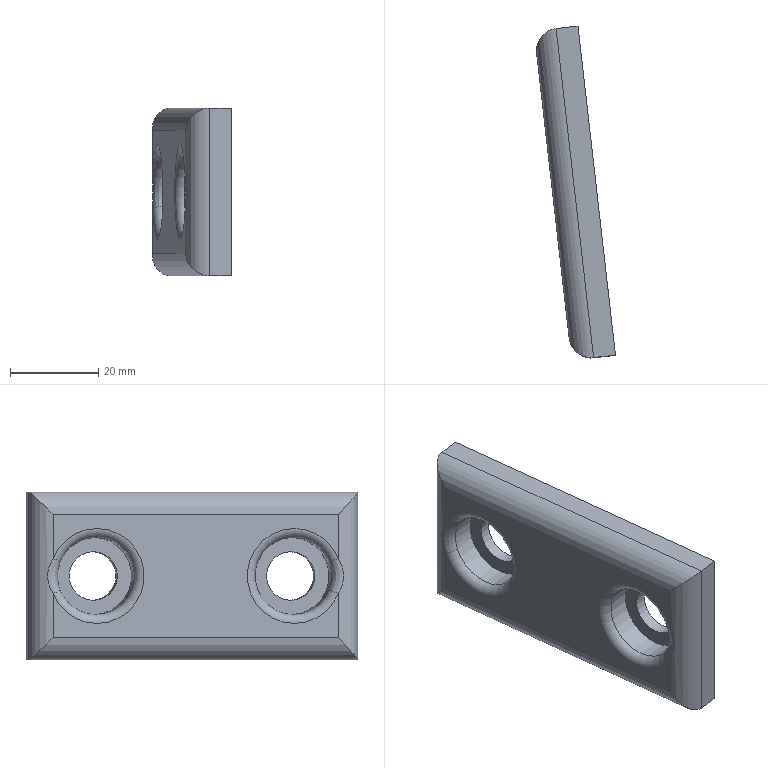Part | NX | features XQ 2 | 1 solid | 20 faces | box 17.898 x 75.116 x 38 mm | volume 23209 mm3 | plane 8 | cylinder 8 | spline 2 | torus 2 | commonest cylinder face diameters 10 x4 11 x2 17.5 x2
STEP:
#1=CARTESIAN_POINT('',(2876.788,318.77,-57.945));
#2=VERTEX_POINT('',#1);
#3=CARTESIAN_POINT('',(2876.788,318.77,-50.055));
#4=VERTEX_POINT('',#3);
#5=CARTESIAN_POINT('',(2876.788,318.77,-50.055));
#6=CARTESIAN_POINT('',(2876.883,317.934,-51.336));
#7=CARTESIAN_POINT('',(2877.291,317.159,-54.001));
#8=CARTESIAN_POINT('',(2876.883,317.934,-56.664));
#9=CARTESIAN_POINT('',(2876.788,318.77,-57.945));
#10=B_SPLINE_CURVE_WITH_KNOTS('',3,(#5,#6,#7,#8,#9),.UNSPECIFIED.,.F.,.F.,(4,1,4),(0.,0.5,1.),.UNSPECIFIED.);
#11=EDGE_CURVE('',#2,#4,#10,.F.);
#12=ORIENTED_EDGE('',*,*,#11,.T.);
#13=CARTESIAN_POINT('',(2878.565,320.845,-50.789));
#14=VERTEX_POINT('',#13);
#15=CARTESIAN_POINT('',(2878.775,318.997,-50.055));
#16=DIRECTION('',(0.04154,-0.3646,-0.9302));
#17=DIRECTION('',(0.,0.931,-0.3649));
#18=AXIS2_PLACEMENT_3D('',#15,#16,#17);
#19=CIRCLE('',#18,2.);
#20=EDGE_CURVE('',#4,#14,#19,.T.);
#21=ORIENTED_EDGE('',*,*,#20,.T.);
#22=CARTESIAN_POINT('',(2878.565,320.845,-57.211));
#23=VERTEX_POINT('',#22);
#24=CARTESIAN_POINT('',(2878.565,320.845,-57.211));
#25=CARTESIAN_POINT('',(2878.572,320.778,-57.039));
#26=CARTESIAN_POINT('',(2878.597,320.624,-56.62));
#27=CARTESIAN_POINT('',(2878.666,320.375,-55.639));
#28=CARTESIAN_POINT('',(2878.721,320.257,-54.616));
#29=CARTESIAN_POINT('',(2878.732,320.246,-54.002));
#30=CARTESIAN_POINT('',(2878.721,320.257,-53.387));
#31=CARTESIAN_POINT('',(2878.666,320.374,-52.363));
#32=CARTESIAN_POINT('',(2878.597,320.624,-51.379));
#33=CARTESIAN_POINT('',(2878.572,320.778,-50.96));
#34=CARTESIAN_POINT('',(2878.565,320.845,-50.789));
#35=B_SPLINE_CURVE_WITH_KNOTS('',3,(#24,#25,#26,#27,#28,#29,#30,#31,#32,#33,#34),.UNSPECIFIED.,.F.,.F.,(4,1,1,1,1,1,1,1,4),(0.,0.125,0.25,0.375,0.5,0.625,0.75,0.875,1.),.UNSPECIFIED.);
#36=EDGE_CURVE('',#14,#23,#35,.F.);
#37=ORIENTED_EDGE('',*,*,#36,.T.);
#38=CARTESIAN_POINT('',(2878.775,318.997,-57.945));
#39=DIRECTION('',(0.04154,-0.3646,0.9302));
#40=DIRECTION('',(0.,0.931,0.3649));
#41=AXIS2_PLACEMENT_3D('',#38,#39,#40);
#42=CIRCLE('',#41,2.);
#43=EDGE_CURVE('',#23,#2,#42,.T.);
#44=ORIENTED_EDGE('',*,*,#43,.T.);
#45=EDGE_LOOP('',(#12,#21,#37,#44));
#46=FACE_BOUND('',#45,.T.);
#47=CARTESIAN_POINT('',(2878.565,320.845,-50.789));
#48=CARTESIAN_POINT('',(2876.577,320.619,-50.789));
#49=CARTESIAN_POINT('',(2876.788,318.77,-50.055));
#50=CARTESIAN_POINT('',(2878.61,320.445,-51.812));
#51=CARTESIAN_POINT('',(2876.298,320.092,-52.036));
#52=CARTESIAN_POINT('',(2876.882,317.95,-51.311));
#53=CARTESIAN_POINT('',(2878.728,320.25,-52.902));
#54=CARTESIAN_POINT('',(2876.163,319.957,-52.986));
#55=CARTESIAN_POINT('',(2877.087,317.547,-52.652));
#56=CARTESIAN_POINT('',(2878.728,320.25,-55.096));
#57=CARTESIAN_POINT('',(2876.163,319.957,-55.012));
#58=CARTESIAN_POINT('',(2877.087,317.546,-55.346));
#59=CARTESIAN_POINT('',(2878.61,320.446,-56.192));
#60=CARTESIAN_POINT('',(2876.299,320.094,-55.968));
#61=CARTESIAN_POINT('',(2876.881,317.952,-56.693));
#62=CARTESIAN_POINT('',(2878.565,320.845,-57.211));
#63=CARTESIAN_POINT('',(2876.577,320.619,-57.211));
#64=CARTESIAN_POINT('',(2876.788,318.77,-57.945));
#65=(BOUNDED_SURFACE()B_SPLINE_SURFACE(3,2,((#47,#48,#49),(#50,#51,#52),(#53,#54,#55),(#56,#57,#58),(#59,#60,#61),(#62,#63,#64)),.UNSPECIFIED.,.F.,.F.,.F.)B_SPLINE_SURFACE_WITH_KNOTS((4,2,4),(3,3),(0.,0.5,1.),(0.,1.),.UNSPECIFIED.)GEOMETRIC_REPRESENTATION_ITEM()RATIONAL_B_SPLINE_SURFACE(((1.,0.7071,1.),(1.,0.6518,1.),(1.,0.6124,1.),(1.,0.6124,1.),(1.,0.6519,1.),(1.,0.7071,1.)))REPRESENTATION_ITEM('')SURFACE());
#66=ADVANCED_FACE('',(#46),#65,.T.);
#67=CARTESIAN_POINT('',(2869.43,383.353,-50.055));
#68=VERTEX_POINT('',#67);
#69=CARTESIAN_POINT('',(2869.43,383.353,-57.945));
#70=VERTEX_POINT('',#69);
#71=CARTESIAN_POINT('',(2869.43,383.353,-57.945));
#72=CARTESIAN_POINT('',(2869.335,384.189,-56.664));
#73=CARTESIAN_POINT('',(2869.558,385.036,-53.999));
#74=CARTESIAN_POINT('',(2869.334,384.19,-51.336));
#75=CARTESIAN_POINT('',(2869.43,383.353,-50.055));
#76=B_SPLINE_CURVE_WITH_KNOTS('',3,(#71,#72,#73,#74,#75),.UNSPECIFIED.,.F.,.F.,(4,1,4),(0.,0.5,1.),.UNSPECIFIED.);
#77=EDGE_CURVE('',#68,#70,#76,.F.);
#78=ORIENTED_EDGE('',*,*,#77,.T.);
#79=CARTESIAN_POINT('',(2871.628,381.731,-57.211));
#80=VERTEX_POINT('',#79);
#81=CARTESIAN_POINT('',(2871.417,383.579,-57.945));
#82=DIRECTION('',(-0.04154,0.3646,0.9302));
#83=DIRECTION('',(0.,-0.931,0.3649));
#84=AXIS2_PLACEMENT_3D('',#81,#82,#83);
#85=CIRCLE('',#84,2.);
#86=EDGE_CURVE('',#70,#80,#85,.T.);
#87=ORIENTED_EDGE('',*,*,#86,.T.);
#88=CARTESIAN_POINT('',(2871.628,381.731,-50.789));
#89=VERTEX_POINT('',#88);
#90=CARTESIAN_POINT('',(2871.628,381.731,-50.789));
#91=CARTESIAN_POINT('',(2871.62,381.798,-50.961));
#92=CARTESIAN_POINT('',(2871.609,381.953,-51.38));
#93=CARTESIAN_POINT('',(2871.621,382.212,-52.361));
#94=CARTESIAN_POINT('',(2871.647,382.339,-53.383));
#95=CARTESIAN_POINT('',(2871.656,382.352,-53.998));
#96=CARTESIAN_POINT('',(2871.647,382.339,-54.613));
#97=CARTESIAN_POINT('',(2871.621,382.212,-55.637));
#98=CARTESIAN_POINT('',(2871.609,381.953,-56.621));
#99=CARTESIAN_POINT('',(2871.62,381.798,-57.04));
#100=CARTESIAN_POINT('',(2871.628,381.731,-57.211));
#101=B_SPLINE_CURVE_WITH_KNOTS('',3,(#90,#91,#92,#93,#94,#95,#96,#97,#98,#99,#100),.UNSPECIFIED.,.F.,.F.,(4,1,1,1,1,1,1,1,4),(0.,0.125,0.25,0.375,0.5,0.625,0.75,0.875,1.),.UNSPECIFIED.);
#102=EDGE_CURVE('',#80,#89,#101,.F.);
#103=ORIENTED_EDGE('',*,*,#102,.T.);
#104=CARTESIAN_POINT('',(2871.417,383.579,-50.055));
#105=DIRECTION('',(-0.04154,0.3646,-0.9302));
#106=DIRECTION('',(0.,-0.931,-0.3649));
#107=AXIS2_PLACEMENT_3D('',#104,#105,#106);
#108=CIRCLE('',#107,2.);
#109=EDGE_CURVE('',#89,#68,#108,.T.);
#110=ORIENTED_EDGE('',*,*,#109,.T.);
#111=EDGE_LOOP('',(#78,#87,#103,#110));
#112=FACE_BOUND('',#111,.T.);
#113=CARTESIAN_POINT('',(2871.628,381.731,-57.211));
#114=CARTESIAN_POINT('',(2869.64,381.504,-57.211));
#115=CARTESIAN_POINT('',(2869.43,383.353,-57.945));
#116=CARTESIAN_POINT('',(2871.582,382.131,-56.188));
#117=CARTESIAN_POINT('',(2869.249,381.955,-55.964));
#118=CARTESIAN_POINT('',(2869.336,384.173,-56.689));
#119=CARTESIAN_POINT('',(2871.653,382.348,-55.098));
#120=CARTESIAN_POINT('',(2869.088,382.055,-55.014));
#121=CARTESIAN_POINT('',(2869.446,384.612,-55.348));
#122=CARTESIAN_POINT('',(2871.653,382.348,-52.904));
#123=CARTESIAN_POINT('',(2869.088,382.056,-52.988));
#124=CARTESIAN_POINT('',(2869.446,384.613,-52.654));
#125=CARTESIAN_POINT('',(2871.582,382.13,-51.808));
#126=CARTESIAN_POINT('',(2869.251,381.953,-52.032));
#127=CARTESIAN_POINT('',(2869.337,384.171,-51.307));
#128=CARTESIAN_POINT('',(2871.628,381.731,-50.789));
#129=CARTESIAN_POINT('',(2869.64,381.504,-50.789));
#130=CARTESIAN_POINT('',(2869.43,383.353,-50.055));
#131=(BOUNDED_SURFACE()B_SPLINE_SURFACE(3,2,((#113,#114,#115),(#116,#117,#118),(#119,#120,#121),(#122,#123,#124),(#125,#126,#127),(#128,#129,#130)),.UNSPECIFIED.,.F.,.F.,.F.)B_SPLINE_SURFACE_WITH_KNOTS((4,2,4),(3,3),(0.,0.5,1.),(0.,1.),.UNSPECIFIED.)GEOMETRIC_REPRESENTATION_ITEM()RATIONAL_B_SPLINE_SURFACE(((1.,0.7071,1.),(1.,0.6518,1.),(1.,0.6124,1.),(1.,0.6124,1.),(1.,0.6519,1.),(1.,0.7071,1.)))REPRESENTATION_ITEM('')SURFACE());
#132=ADVANCED_FACE('',(#112),#131,.T.);
#133=CARTESIAN_POINT('',(2882.322,314.369,-73.));
#134=VERTEX_POINT('',#133);
#135=CARTESIAN_POINT('',(2887.29,314.935,-73.));
#136=VERTEX_POINT('',#135);
#137=CARTESIAN_POINT('',(2882.322,314.369,-73.));
#138=DIRECTION('',(0.9936,0.1132,0.000000001));
#139=VECTOR('',#138,1000.);
#140=LINE('',#137,#139);
#141=EDGE_CURVE('',#134,#136,#140,.T.);
#142=ORIENTED_EDGE('',*,*,#141,.T.);
#143=CARTESIAN_POINT('',(2887.29,314.935,-35.));
#144=VERTEX_POINT('',#143);
#145=CARTESIAN_POINT('',(2887.29,314.935,-59.));
#146=DIRECTION('',(0.000000001,0.,-1.));
#147=VECTOR('',#146,1000.);
#148=LINE('',#145,#147);
#149=EDGE_CURVE('',#144,#136,#148,.T.);
#150=ORIENTED_EDGE('',*,*,#149,.F.);
#151=CARTESIAN_POINT('',(2882.322,314.369,-35.));
#152=VERTEX_POINT('',#151);
#153=CARTESIAN_POINT('',(2882.322,314.369,-35.));
#154=DIRECTION('',(-0.9936,-0.1132,-0.000000001));
#155=VECTOR('',#154,1000.);
#156=LINE('',#153,#155);
#157=EDGE_CURVE('',#144,#152,#156,.T.);
#158=ORIENTED_EDGE('',*,*,#157,.T.);
#159=CARTESIAN_POINT('',(2882.322,314.369,-54.));
#160=DIRECTION('',(0.000000001,0.,-1.));
#161=VECTOR('',#160,1000.);
#162=LINE('',#159,#161);
#163=EDGE_CURVE('',#152,#134,#162,.T.);
#164=ORIENTED_EDGE('',*,*,#163,.T.);
#165=EDGE_LOOP('',(#142,#150,#158,#164));
#166=FACE_BOUND('',#165,.T.);
#167=CARTESIAN_POINT('',(2882.322,314.369,-59.));
#168=DIRECTION('',(-0.1132,0.9936,0.));
#169=DIRECTION('',(-0.9936,-0.1132,-0.000000001));
#170=AXIS2_PLACEMENT_3D('',#167,#168,#169);
#171=PLANE('',#170);
#172=ADVANCED_FACE('',(#166),#171,.F.);
#173=CARTESIAN_POINT('',(2878.8,389.453,-73.));
#174=VERTEX_POINT('',#173);
#175=CARTESIAN_POINT('',(2873.832,388.887,-73.));
#176=VERTEX_POINT('',#175);
#177=CARTESIAN_POINT('',(2873.832,388.887,-73.));
#178=DIRECTION('',(-0.9936,-0.1132,-0.000000001));
#179=VECTOR('',#178,1000.);
#180=LINE('',#177,#179);
#181=EDGE_CURVE('',#174,#176,#180,.T.);
#182=ORIENTED_EDGE('',*,*,#181,.F.);
#183=CARTESIAN_POINT('',(2885.875,327.354,-73.));
#184=DIRECTION('',(-0.1132,0.9936,0.));
#185=VECTOR('',#184,1000.);
#186=LINE('',#183,#185);
#187=EDGE_CURVE('',#136,#174,#186,.T.);
#188=ORIENTED_EDGE('',*,*,#187,.F.);
#189=ORIENTED_EDGE('',*,*,#141,.F.);
#190=CARTESIAN_POINT('',(2875.247,376.467,-73.));
#191=DIRECTION('',(-0.1132,0.9936,0.));
#192=VECTOR('',#191,1000.);
#193=LINE('',#190,#192);
#194=EDGE_CURVE('',#134,#176,#193,.T.);
#195=ORIENTED_EDGE('',*,*,#194,.T.);
#196=EDGE_LOOP('',(#182,#188,#189,#195));
#197=FACE_BOUND('',#196,.T.);
#198=CARTESIAN_POINT('',(2880.907,326.788,-73.));
#199=DIRECTION('',(-0.000000001,0.,1.));
#200=DIRECTION('',(-0.9936,-0.1132,-0.000000001));
#201=AXIS2_PLACEMENT_3D('',#198,#199,#200);
#202=PLANE('',#201);
#203=ADVANCED_FACE('',(#197),#202,.F.);
#204=ORIENTED_EDGE('',*,*,#194,.F.);
#205=CARTESIAN_POINT('',(2876.788,318.77,-68.));
#206=VERTEX_POINT('',#205);
#207=CARTESIAN_POINT('',(2881.756,319.336,-68.));
#208=DIRECTION('',(0.08005,-0.7026,0.7071));
#209=DIRECTION('',(-0.08005,0.7026,0.7071));
#210=AXIS2_PLACEMENT_3D('',#207,#208,#209);
#211=ELLIPSE('',#210,7.071,5.);
#212=EDGE_CURVE('',#206,#134,#211,.T.);
#213=ORIENTED_EDGE('',*,*,#212,.F.);
#214=CARTESIAN_POINT('',(2869.43,383.353,-68.));
#215=VERTEX_POINT('',#214);
#216=CARTESIAN_POINT('',(2870.279,375.901,-68.));
#217=DIRECTION('',(0.1132,-0.9936,0.));
#218=VECTOR('',#217,1000.);
#219=LINE('',#216,#218);
#220=EDGE_CURVE('',#215,#206,#219,.T.);
#221=ORIENTED_EDGE('',*,*,#220,.F.);
#222=CARTESIAN_POINT('',(2874.398,383.919,-68.));
#223=DIRECTION('',(0.08005,-0.7026,-0.7071));
#224=DIRECTION('',(0.08005,-0.7026,0.7071));
#225=AXIS2_PLACEMENT_3D('',#222,#223,#224);
#226=ELLIPSE('',#225,7.071,5.);
#227=EDGE_CURVE('',#215,#176,#226,.T.);
#228=ORIENTED_EDGE('',*,*,#227,.T.);
#229=EDGE_LOOP('',(#204,#213,#221,#228));
#230=FACE_BOUND('',#229,.T.);
#231=CARTESIAN_POINT('',(2875.247,376.467,-68.));
#232=DIRECTION('',(-0.1132,0.9936,0.));
#233=DIRECTION('',(-0.7026,-0.08005,-0.7071));
#234=AXIS2_PLACEMENT_3D('',#231,#232,#233);
#235=CYLINDRICAL_SURFACE('',#234,5.);
#236=ADVANCED_FACE('',(#230),#235,.T.);
#237=ORIENTED_EDGE('',*,*,#157,.F.);
#238=CARTESIAN_POINT('',(2878.8,389.453,-35.));
#239=VERTEX_POINT('',#238);
#240=CARTESIAN_POINT('',(2885.875,327.354,-35.));
#241=DIRECTION('',(0.1132,-0.9936,0.));
#242=VECTOR('',#241,1000.);
#243=LINE('',#240,#242);
#244=EDGE_CURVE('',#239,#144,#243,.T.);
#245=ORIENTED_EDGE('',*,*,#244,.F.);
#246=CARTESIAN_POINT('',(2873.832,388.887,-35.));
#247=VERTEX_POINT('',#246);
#248=CARTESIAN_POINT('',(2873.832,388.887,-35.));
#249=DIRECTION('',(0.9936,0.1132,0.000000001));
#250=VECTOR('',#249,1000.);
#251=LINE('',#248,#250);
#252=EDGE_CURVE('',#247,#239,#251,.T.);
#253=ORIENTED_EDGE('',*,*,#252,.F.);
#254=CARTESIAN_POINT('',(2875.247,376.467,-35.));
#255=DIRECTION('',(0.1132,-0.9936,0.));
#256=VECTOR('',#255,1000.);
#257=LINE('',#254,#256);
#258=EDGE_CURVE('',#247,#152,#257,.T.);
#259=ORIENTED_EDGE('',*,*,#258,.T.);
#260=EDGE_LOOP('',(#237,#245,#253,#259));
#261=FACE_BOUND('',#260,.T.);
#262=CARTESIAN_POINT('',(2880.907,326.788,-35.));
#263=DIRECTION('',(0.000000001,0.,-1.));
#264=DIRECTION('',(0.9936,0.1132,0.000000001));
#265=AXIS2_PLACEMENT_3D('',#262,#263,#264);
#266=PLANE('',#265);
#267=ADVANCED_FACE('',(#261),#266,.F.);
#268=CARTESIAN_POINT('',(2876.788,318.77,-40.));
#269=VERTEX_POINT('',#268);
#270=CARTESIAN_POINT('',(2869.43,383.353,-40.));
#271=VERTEX_POINT('',#270);
#272=CARTESIAN_POINT('',(2870.279,375.901,-40.));
#273=DIRECTION('',(-0.1132,0.9936,0.));
#274=VECTOR('',#273,1000.);
#275=LINE('',#272,#274);
#276=EDGE_CURVE('',#269,#271,#275,.T.);
#277=ORIENTED_EDGE('',*,*,#276,.F.);
#278=CARTESIAN_POINT('',(2881.756,319.336,-40.));
#279=DIRECTION('',(-0.08005,0.7026,0.7071));
#280=DIRECTION('',(-0.08005,0.7026,-0.7071));
#281=AXIS2_PLACEMENT_3D('',#278,#279,#280);
#282=ELLIPSE('',#281,7.071,5.);
#283=EDGE_CURVE('',#269,#152,#282,.T.);
#284=ORIENTED_EDGE('',*,*,#283,.T.);
#285=ORIENTED_EDGE('',*,*,#258,.F.);
#286=CARTESIAN_POINT('',(2874.398,383.919,-40.));
#287=DIRECTION('',(-0.08005,0.7026,-0.7071));
#288=DIRECTION('',(0.08005,-0.7026,-0.7071));
#289=AXIS2_PLACEMENT_3D('',#286,#287,#288);
#290=ELLIPSE('',#289,7.071,5.);
#291=EDGE_CURVE('',#271,#247,#290,.T.);
#292=ORIENTED_EDGE('',*,*,#291,.F.);
#293=EDGE_LOOP('',(#277,#284,#285,#292));
#294=FACE_BOUND('',#293,.T.);
#295=CARTESIAN_POINT('',(2875.247,376.467,-40.));
#296=DIRECTION('',(0.1132,-0.9936,0.));
#297=DIRECTION('',(-0.7026,-0.08005,0.7071));
#298=AXIS2_PLACEMENT_3D('',#295,#296,#297);
#299=CYLINDRICAL_SURFACE('',#298,5.);
#300=ADVANCED_FACE('',(#294),#299,.T.);
#301=CARTESIAN_POINT('',(2876.788,318.77,-54.));
#302=DIRECTION('',(-0.000000001,0.,1.));
#303=VECTOR('',#302,1000.);
#304=LINE('',#301,#303);
#305=EDGE_CURVE('',#206,#2,#304,.T.);
#306=ORIENTED_EDGE('',*,*,#305,.F.);
#307=ORIENTED_EDGE('',*,*,#212,.T.);
#308=ORIENTED_EDGE('',*,*,#163,.F.);
#309=ORIENTED_EDGE('',*,*,#283,.F.);
#310=CARTESIAN_POINT('',(2876.788,318.77,-54.));
#311=DIRECTION('',(-0.000000001,0.,1.));
#312=VECTOR('',#311,1000.);
#313=LINE('',#310,#312);
#314=EDGE_CURVE('',#4,#269,#313,.T.);
#315=ORIENTED_EDGE('',*,*,#314,.F.);
#316=ORIENTED_EDGE('',*,*,#11,.F.);
#317=EDGE_LOOP('',(#306,#307,#308,#309,#315,#316));
#318=FACE_BOUND('',#317,.T.);
#319=CARTESIAN_POINT('',(2881.756,319.336,-54.));
#320=DIRECTION('',(0.000000001,0.,-1.));
#321=DIRECTION('',(-0.6225,-0.7826,0.));
#322=AXIS2_PLACEMENT_3D('',#319,#320,#321);
#323=CYLINDRICAL_SURFACE('',#322,5.);
#324=ADVANCED_FACE('',(#318),#323,.T.);
#325=CARTESIAN_POINT('',(2869.43,383.353,-54.));
#326=DIRECTION('',(0.000000001,0.,-1.));
#327=VECTOR('',#326,1000.);
#328=LINE('',#325,#327);
#329=EDGE_CURVE('',#271,#68,#328,.T.);
#330=ORIENTED_EDGE('',*,*,#329,.F.);
#331=ORIENTED_EDGE('',*,*,#291,.T.);
#332=CARTESIAN_POINT('',(2873.832,388.887,-54.));
#333=DIRECTION('',(-0.000000001,0.,1.));
#334=VECTOR('',#333,1000.);
#335=LINE('',#332,#334);
#336=EDGE_CURVE('',#176,#247,#335,.T.);
#337=ORIENTED_EDGE('',*,*,#336,.F.);
#338=ORIENTED_EDGE('',*,*,#227,.F.);
#339=CARTESIAN_POINT('',(2869.43,383.353,-54.));
#340=DIRECTION('',(0.000000001,0.,-1.));
#341=VECTOR('',#340,1000.);
#342=LINE('',#339,#341);
#343=EDGE_CURVE('',#70,#215,#342,.T.);
#344=ORIENTED_EDGE('',*,*,#343,.F.);
#345=ORIENTED_EDGE('',*,*,#77,.F.);
#346=EDGE_LOOP('',(#330,#331,#337,#338,#344,#345));
#347=FACE_BOUND('',#346,.T.);
#348=CARTESIAN_POINT('',(2874.398,383.919,-54.));
#349=DIRECTION('',(-0.000000001,0.,1.));
#350=DIRECTION('',(-0.7826,0.6225,-0.000000001));
#351=AXIS2_PLACEMENT_3D('',#348,#349,#350);
#352=CYLINDRICAL_SURFACE('',#351,5.);
#353=ADVANCED_FACE('',(#347),#352,.T.);
#354=CARTESIAN_POINT('',(2875.656,328.706,-64.75));
#355=VERTEX_POINT('',#354);
#356=CARTESIAN_POINT('',(2875.656,328.706,-54.));
#357=DIRECTION('',(0.9936,0.1132,0.000000001));
#358=DIRECTION('',(-0.000000001,0.,1.));
#359=AXIS2_PLACEMENT_3D('',#356,#357,#358);
#360=CIRCLE('',#359,10.75);
#361=EDGE_CURVE('',#2,#355,#360,.T.);
#362=ORIENTED_EDGE('',*,*,#361,.T.);
#363=CARTESIAN_POINT('',(2875.656,328.706,-54.));
#364=DIRECTION('',(0.9936,0.1132,0.000000001));
#365=DIRECTION('',(-0.000000001,0.,1.));
#366=AXIS2_PLACEMENT_3D('',#363,#364,#365);
#367=CIRCLE('',#366,10.75);
#368=EDGE_CURVE('',#355,#4,#367,.T.);
#369=ORIENTED_EDGE('',*,*,#368,.T.);
#370=ORIENTED_EDGE('',*,*,#314,.T.);
#371=ORIENTED_EDGE('',*,*,#276,.T.);
#372=ORIENTED_EDGE('',*,*,#329,.T.);
#373=CARTESIAN_POINT('',(2870.562,373.417,-54.));
#374=DIRECTION('',(0.9936,0.1132,0.000000001));
#375=DIRECTION('',(-0.1132,0.9936,0.));
#376=AXIS2_PLACEMENT_3D('',#373,#374,#375);
#377=CIRCLE('',#376,10.75);
#378=EDGE_CURVE('',#68,#70,#377,.T.);
#379=ORIENTED_EDGE('',*,*,#378,.T.);
#380=ORIENTED_EDGE('',*,*,#343,.T.);
#381=ORIENTED_EDGE('',*,*,#220,.T.);
#382=ORIENTED_EDGE('',*,*,#305,.T.);
#383=EDGE_LOOP('',(#362,#369,#370,#371,#372,#379,#380,#381,#382));
#384=FACE_BOUND('',#383,.T.);
#385=CARTESIAN_POINT('',(2870.279,375.901,-54.));
#386=DIRECTION('',(-0.9936,-0.1132,-0.000000001));
#387=DIRECTION('',(0.000000001,0.,-1.));
#388=AXIS2_PLACEMENT_3D('',#385,#386,#387);
#389=PLANE('',#388);
#390=ADVANCED_FACE('',(#384),#389,.T.);
#391=ORIENTED_EDGE('',*,*,#149,.T.);
#392=ORIENTED_EDGE('',*,*,#187,.T.);
#393=CARTESIAN_POINT('',(2878.8,389.453,-59.));
#394=DIRECTION('',(0.000000001,0.,-1.));
#395=VECTOR('',#394,1000.);
#396=LINE('',#393,#395);
#397=EDGE_CURVE('',#239,#174,#396,.T.);
#398=ORIENTED_EDGE('',*,*,#397,.F.);
#399=ORIENTED_EDGE('',*,*,#244,.T.);
#400=EDGE_LOOP('',(#391,#392,#398,#399));
#401=FACE_BOUND('',#400,.T.);
#402=CARTESIAN_POINT('',(2885.592,329.838,-59.5));
#403=VERTEX_POINT('',#402);
#404=CARTESIAN_POINT('',(2885.592,329.838,-54.));
#405=DIRECTION('',(0.9936,0.1132,0.000000001));
#406=DIRECTION('',(0.000000001,0.,-1.));
#407=AXIS2_PLACEMENT_3D('',#404,#405,#406);
#408=CIRCLE('',#407,5.5);
#409=EDGE_CURVE('',#403,#403,#408,.T.);
#410=ORIENTED_EDGE('',*,*,#409,.F.);
#411=EDGE_LOOP('',(#410));
#412=FACE_BOUND('',#411,.T.);
#413=CARTESIAN_POINT('',(2880.498,374.549,-59.5));
#414=VERTEX_POINT('',#413);
#415=CARTESIAN_POINT('',(2880.498,374.549,-54.));
#416=DIRECTION('',(0.9936,0.1132,0.000000001));
#417=DIRECTION('',(0.000000001,0.,-1.));
#418=AXIS2_PLACEMENT_3D('',#415,#416,#417);
#419=CIRCLE('',#418,5.5);
#420=EDGE_CURVE('',#414,#414,#419,.T.);
#421=ORIENTED_EDGE('',*,*,#420,.F.);
#422=EDGE_LOOP('',(#421));
#423=FACE_BOUND('',#422,.T.);
#424=CARTESIAN_POINT('',(2885.875,327.354,-59.));
#425=DIRECTION('',(-0.9936,-0.1132,-0.000000001));
#426=DIRECTION('',(0.000000001,0.,-1.));
#427=AXIS2_PLACEMENT_3D('',#424,#425,#426);
#428=PLANE('',#427);
#429=ADVANCED_FACE('',(#401,#412,#423),#428,.F.);
#430=CARTESIAN_POINT('',(2872.549,373.643,-62.75));
#431=VERTEX_POINT('',#430);
#432=CARTESIAN_POINT('',(2872.549,373.643,-54.));
#433=DIRECTION('',(-0.9936,-0.1132,-0.000000001));
#434=DIRECTION('',(-0.000000001,0.,1.));
#435=AXIS2_PLACEMENT_3D('',#432,#433,#434);
#436=CIRCLE('',#435,8.75);
#437=EDGE_CURVE('',#431,#89,#436,.T.);
#438=ORIENTED_EDGE('',*,*,#437,.F.);
#439=CARTESIAN_POINT('',(2872.549,373.643,-54.));
#440=DIRECTION('',(-0.9936,-0.1132,-0.000000001));
#441=DIRECTION('',(-0.000000001,0.,1.));
#442=AXIS2_PLACEMENT_3D('',#439,#440,#441);
#443=CIRCLE('',#442,8.75);
#444=EDGE_CURVE('',#80,#431,#443,.T.);
#445=ORIENTED_EDGE('',*,*,#444,.F.);
#446=ORIENTED_EDGE('',*,*,#86,.F.);
#447=ORIENTED_EDGE('',*,*,#378,.F.);
#448=ORIENTED_EDGE('',*,*,#109,.F.);
#449=EDGE_LOOP('',(#438,#445,#446,#447,#448));
#450=FACE_BOUND('',#449,.T.);
#451=CARTESIAN_POINT('',(2872.549,373.643,-54.));
#452=DIRECTION('',(0.9936,0.1132,0.000000001));
#453=DIRECTION('',(-0.000000001,0.,1.));
#454=AXIS2_PLACEMENT_3D('',#451,#452,#453);
#455=TOROIDAL_SURFACE('',#454,10.75,2.);
#456=ADVANCED_FACE('',(#450),#455,.T.);
#457=CARTESIAN_POINT('',(2877.815,374.243,-62.75));
#458=VERTEX_POINT('',#457);
#459=CARTESIAN_POINT('',(2877.815,374.243,-54.));
#460=DIRECTION('',(-0.9936,-0.1132,-0.000000001));
#461=DIRECTION('',(0.000000001,0.,-1.));
#462=AXIS2_PLACEMENT_3D('',#459,#460,#461);
#463=CIRCLE('',#462,8.75);
#464=EDGE_CURVE('',#458,#458,#463,.T.);
#465=ORIENTED_EDGE('',*,*,#464,.F.);
#466=EDGE_LOOP('',(#465));
#467=FACE_BOUND('',#466,.T.);
#468=ORIENTED_EDGE('',*,*,#444,.T.);
#469=ORIENTED_EDGE('',*,*,#437,.T.);
#470=ORIENTED_EDGE('',*,*,#102,.F.);
#471=EDGE_LOOP('',(#468,#469,#470));
#472=FACE_BOUND('',#471,.T.);
#473=CARTESIAN_POINT('',(2874.188,373.83,-54.));
#474=DIRECTION('',(-0.9936,-0.1132,-0.000000001));
#475=DIRECTION('',(0.000000001,0.,-1.));
#476=AXIS2_PLACEMENT_3D('',#473,#474,#475);
#477=CYLINDRICAL_SURFACE('',#476,8.75);
#478=ADVANCED_FACE('',(#467,#472),#477,.F.);
#479=CARTESIAN_POINT('',(2877.643,328.933,-62.75));
#480=VERTEX_POINT('',#479);
#481=CARTESIAN_POINT('',(2877.643,328.933,-54.));
#482=DIRECTION('',(-0.9936,-0.1132,-0.000000001));
#483=DIRECTION('',(-0.000000001,0.,1.));
#484=AXIS2_PLACEMENT_3D('',#481,#482,#483);
#485=CIRCLE('',#484,8.75);
#486=EDGE_CURVE('',#480,#23,#485,.T.);
#487=ORIENTED_EDGE('',*,*,#486,.F.);
#488=CARTESIAN_POINT('',(2877.643,328.933,-54.));
#489=DIRECTION('',(-0.9936,-0.1132,-0.000000001));
#490=DIRECTION('',(-0.000000001,0.,1.));
#491=AXIS2_PLACEMENT_3D('',#488,#489,#490);
#492=CIRCLE('',#491,8.75);
#493=EDGE_CURVE('',#14,#480,#492,.T.);
#494=ORIENTED_EDGE('',*,*,#493,.F.);
#495=ORIENTED_EDGE('',*,*,#20,.F.);
#496=ORIENTED_EDGE('',*,*,#368,.F.);
#497=ORIENTED_EDGE('',*,*,#361,.F.);
#498=ORIENTED_EDGE('',*,*,#43,.F.);
#499=EDGE_LOOP('',(#487,#494,#495,#496,#497,#498));
#500=FACE_BOUND('',#499,.T.);
#501=CARTESIAN_POINT('',(2877.643,328.933,-54.));
#502=DIRECTION('',(0.9936,0.1132,0.000000001));
#503=DIRECTION('',(-0.000000001,0.,1.));
#504=AXIS2_PLACEMENT_3D('',#501,#502,#503);
#505=TOROIDAL_SURFACE('',#504,10.75,2.);
#506=ADVANCED_FACE('',(#500),#505,.T.);
#507=CARTESIAN_POINT('',(2882.909,329.533,-62.75));
#508=VERTEX_POINT('',#507);
#509=CARTESIAN_POINT('',(2882.909,329.533,-54.));
#510=DIRECTION('',(-0.9936,-0.1132,-0.000000001));
#511=DIRECTION('',(0.000000001,0.,-1.));
#512=AXIS2_PLACEMENT_3D('',#509,#510,#511);
#513=CIRCLE('',#512,8.75);
#514=EDGE_CURVE('',#508,#508,#513,.T.);
#515=ORIENTED_EDGE('',*,*,#514,.F.);
#516=EDGE_LOOP('',(#515));
#517=FACE_BOUND('',#516,.T.);
#518=ORIENTED_EDGE('',*,*,#493,.T.);
#519=ORIENTED_EDGE('',*,*,#486,.T.);
#520=ORIENTED_EDGE('',*,*,#36,.F.);
#521=EDGE_LOOP('',(#518,#519,#520));
#522=FACE_BOUND('',#521,.T.);
#523=CARTESIAN_POINT('',(2879.283,329.119,-54.));
#524=DIRECTION('',(-0.9936,-0.1132,-0.000000001));
#525=DIRECTION('',(0.000000001,0.,-1.));
#526=AXIS2_PLACEMENT_3D('',#523,#524,#525);
#527=CYLINDRICAL_SURFACE('',#526,8.75);
#528=ADVANCED_FACE('',(#517,#522),#527,.F.);
#529=ORIENTED_EDGE('',*,*,#420,.T.);
#530=EDGE_LOOP('',(#529));
#531=FACE_BOUND('',#530,.T.);
#532=CARTESIAN_POINT('',(2877.815,374.243,-59.5));
#533=VERTEX_POINT('',#532);
#534=CARTESIAN_POINT('',(2877.815,374.243,-54.));
#535=DIRECTION('',(0.9936,0.1132,0.000000001));
#536=DIRECTION('',(0.000000001,0.,-1.));
#537=AXIS2_PLACEMENT_3D('',#534,#535,#536);
#538=CIRCLE('',#537,5.5);
#539=EDGE_CURVE('',#533,#533,#538,.T.);
#540=ORIENTED_EDGE('',*,*,#539,.F.);
#541=EDGE_LOOP('',(#540));
#542=FACE_BOUND('',#541,.T.);
#543=CARTESIAN_POINT('',(2879.156,374.396,-54.));
#544=DIRECTION('',(-0.9936,-0.1132,-0.000000001));
#545=DIRECTION('',(0.000000001,0.,-1.));
#546=AXIS2_PLACEMENT_3D('',#543,#544,#545);
#547=CYLINDRICAL_SURFACE('',#546,5.5);
#548=ADVANCED_FACE('',(#531,#542),#547,.F.);
#549=ORIENTED_EDGE('',*,*,#539,.T.);
#550=EDGE_LOOP('',(#549));
#551=FACE_BOUND('',#550,.T.);
#552=ORIENTED_EDGE('',*,*,#464,.T.);
#553=EDGE_LOOP('',(#552));
#554=FACE_BOUND('',#553,.T.);
#555=CARTESIAN_POINT('',(2877.815,374.243,-54.));
#556=DIRECTION('',(0.9936,0.1132,0.000000001));
#557=DIRECTION('',(-0.000000001,0.,1.));
#558=AXIS2_PLACEMENT_3D('',#555,#556,#557);
#559=PLANE('',#558);
#560=ADVANCED_FACE('',(#551,#554),#559,.F.);
#561=ORIENTED_EDGE('',*,*,#409,.T.);
#562=EDGE_LOOP('',(#561));
#563=FACE_BOUND('',#562,.T.);
#564=CARTESIAN_POINT('',(2882.909,329.533,-59.5));
#565=VERTEX_POINT('',#564);
#566=CARTESIAN_POINT('',(2882.909,329.533,-54.));
#567=DIRECTION('',(0.9936,0.1132,0.000000001));
#568=DIRECTION('',(0.000000001,0.,-1.));
#569=AXIS2_PLACEMENT_3D('',#566,#567,#568);
#570=CIRCLE('',#569,5.5);
#571=EDGE_CURVE('',#565,#565,#570,.T.);
#572=ORIENTED_EDGE('',*,*,#571,.F.);
#573=EDGE_LOOP('',(#572));
#574=FACE_BOUND('',#573,.T.);
#575=CARTESIAN_POINT('',(2884.25,329.685,-54.));
#576=DIRECTION('',(-0.9936,-0.1132,-0.000000001));
#577=DIRECTION('',(0.000000001,0.,-1.));
#578=AXIS2_PLACEMENT_3D('',#575,#576,#577);
#579=CYLINDRICAL_SURFACE('',#578,5.5);
#580=ADVANCED_FACE('',(#563,#574),#579,.F.);
#581=ORIENTED_EDGE('',*,*,#571,.T.);
#582=EDGE_LOOP('',(#581));
#583=FACE_BOUND('',#582,.T.);
#584=ORIENTED_EDGE('',*,*,#514,.T.);
#585=EDGE_LOOP('',(#584));
#586=FACE_BOUND('',#585,.T.);
#587=CARTESIAN_POINT('',(2882.909,329.533,-54.));
#588=DIRECTION('',(0.9936,0.1132,0.000000001));
#589=DIRECTION('',(-0.000000001,0.,1.));
#590=AXIS2_PLACEMENT_3D('',#587,#588,#589);
#591=PLANE('',#590);
#592=ADVANCED_FACE('',(#583,#586),#591,.F.);
#593=ORIENTED_EDGE('',*,*,#336,.T.);
#594=ORIENTED_EDGE('',*,*,#252,.T.);
#595=ORIENTED_EDGE('',*,*,#397,.T.);
#596=ORIENTED_EDGE('',*,*,#181,.T.);
#597=EDGE_LOOP('',(#593,#594,#595,#596));
#598=FACE_BOUND('',#597,.T.);
#599=CARTESIAN_POINT('',(2873.832,388.887,-59.));
#600=DIRECTION('',(0.1132,-0.9936,0.));
#601=DIRECTION('',(0.9936,0.1132,0.000000001));
#602=AXIS2_PLACEMENT_3D('',#599,#600,#601);
#603=PLANE('',#602);
#604=ADVANCED_FACE('',(#598),#603,.F.);
#605=CLOSED_SHELL('',(#66,#132,#172,#203,#236,#267,#300,#324,#353,#390,#429,#456,#478,#506,#528,#548,#560,#580,#592,#604));
#606=MANIFOLD_SOLID_BREP('',#605);
#607=(LENGTH_UNIT()NAMED_UNIT(*)SI_UNIT(.MILLI.,.METRE.));
#608=UNCERTAINTY_MEASURE_WITH_UNIT(LENGTH_MEASURE(0.0508),#607,'','');
#609=(NAMED_UNIT(*)PLANE_ANGLE_UNIT()SI_UNIT($,.RADIAN.));
#610=(NAMED_UNIT(*)SI_UNIT($,.STERADIAN.)SOLID_ANGLE_UNIT());
#611=(GEOMETRIC_REPRESENTATION_CONTEXT(3)GLOBAL_UNCERTAINTY_ASSIGNED_CONTEXT((#608))GLOBAL_UNIT_ASSIGNED_CONTEXT((#607,#609,#610))REPRESENTATION_CONTEXT('',''));
#612=ADVANCED_BREP_SHAPE_REPRESENTATION('',(#606),#611);